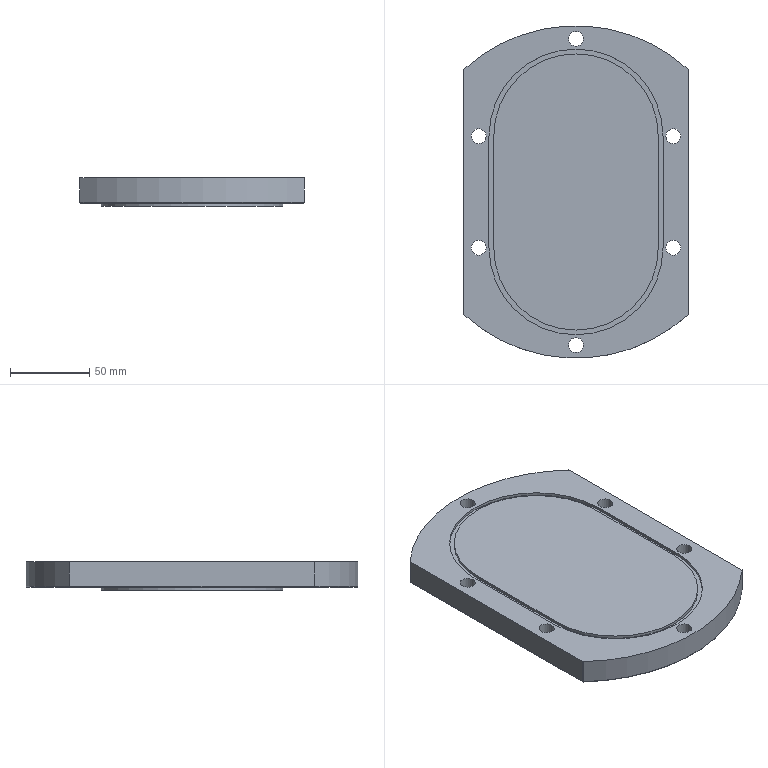NC program | NX | posted with a generic post | part box 142 x 210 x 18 mm
Whole program, first 1636 of 1921 lines:
N10 G17 G21 G94 G90
(FLOOR_WALL_COPY_1 , TOOL : D50)
N12 T02 M6
N14 G54
N16 G17 G0 G90 X-85.265 Y114.816 S1200 M3
N18 G43 Z30. H2
N20 Z7.65
N22 G94 G1 Z4.65 F1000.
N24 X-80.13
N26 X80.117 F2000.
N28 G2 X82.943 Y112.789 R139.395
N30 X115.013 Y79.847 R139.657
N32 G1 X-115.005
N34 G3 X-132.614 Y44.877 R139.395
N36 G1 X132.619
N38 G2 X135.762 Y34.188 R138.402
N40 X138.212 Y22.319 R138.876
N42 X139.185 Y15.081 R138.848
N44 G1 X139.188 Y15.055
N46 G2 X139.52 Y11.62 R138.455
N48 X139.654 Y9.908 R139.238
N50 G1 X-139.654
N52 G3 X-140. Y1.556 R138.451
N54 G1 Y-1.551
N56 G3 X-139.185 Y-15.081 R138.451
N58 X-139.096 Y-15.879 R138.876
N60 X-137.742 Y-25.061 R138.874
N62 G1 X137.753
N64 G2 X133.543 Y-42.026 R139.238
N66 G1 X133.535 Y-42.053
N68 G2 X126.487 Y-60.031 R139.394
N70 G1 X-126.475
N72 G3 X-102.857 Y-95. R139.108
N74 G1 X102.85
N76 X106.896
N78 Z7.65
N80 G0 Z30.
N82 X-85.278 Y114.807
N84 Z7.3
N86 G1 Z4.3 F1000.
N88 X-80.144
N90 X80.131 F2000.
N92 G2 X82.943 Y112.789 R139.395
N94 X88.4 Y108.57 R139.657
N96 X95.762 Y102.141 R139.226
N98 X115.019 Y79.839 R139.657
N100 G1 X-115.01
N102 G3 X-131.183 Y48.912 R139.395
N104 X-132.617 Y44.871 R139.232
N106 G1 X132.621
N108 G2 X133.663 Y41.664 R138.402
N110 X138.725 Y18.859 R139.471
N112 X139.177 Y15.15 R138.876
N114 X139.284 Y14.148 R138.613
N116 X139.654 Y9.903 R138.455
N118 G1 X-139.654
N120 G3 X-140. Y1.556 R138.452
N122 G1 Y-1.551
N124 G3 X-139.284 Y-14.144 R138.452
N126 X-139.177 Y-15.15 R138.609
N128 X-138.72 Y-18.899 R138.874
N130 X-137.742 Y-25.064 R139.469
N132 G1 X137.744
N134 G2 X133.556 Y-41.985 R138.547
N136 X131.173 Y-48.938 R139.231
N138 X126.486 Y-60.032 R139.394
N140 G1 X-126.494
N142 G3 X-102.838 Y-95. R140.983
N144 G1 X102.85
N146 X106.897
N148 Z7.3
N150 G0 Z30.
N152 X-85.269 Y114.807
N154 Z6.95
N156 G1 Z3.95 F1000.
N158 X-80.13
N160 X80.121 F2000.
N162 G2 X115.009 Y79.839 R139.149
N164 G1 X-115.002
N166 G3 X-115.739 Y78.769 R139.74
N168 X-128.743 Y55.02 R139.232
N170 X-132.622 Y44.871 R139.74
N172 G1 X132.62
N174 G2 X135.313 Y35.943 R139.471
N176 X139.159 Y15.32 R137.837
N178 X139.414 Y12.819 R138.939
N180 X139.653 Y9.903 R138.613
N182 G1 X-139.654
N184 G3 X-140. Y1.469 R138.609
N186 G1 Y-1.466
N188 G3 X-139.415 Y-12.808 R138.609
N190 X-139.159 Y-15.32 R138.939
N192 X-137.747 Y-25.064 R137.838
N194 G1 X137.742
N196 G2 X128.804 Y-54.879 R139.741
N198 X126.485 Y-60.032 R139.231
N200 G1 X-126.494
N202 G3 X-122.148 Y-68.39 R123.247
N204 X-118.721 Y-74.228 R123.999
N206 X-113.449 Y-82.027 R127.339
N208 X-103.593 Y-94.179 R130.009
N210 X-102.842 Y-95. R138.664
N212 G1 X102.854
N214 X106.901
N216 Z6.95
N218 G0 Z30.
N220 X-85.269 Y114.807
N222 Z6.6
N224 G1 Z3.6 F1000.
N226 X-80.13
N228 X80.122 F2000.
N230 G2 X83.799 Y112.156 R139.171
N232 X115.009 Y79.839 R139.149
N234 G1 X-115.003
N236 X-115.016 Y79.82
N238 G3 X-124.925 Y63.209 R138.142
N240 X-132.622 Y44.871 R139.74
N242 G1 X132.617
N244 G2 X133.643 Y41.704 R137.21
N246 X134.529 Y38.766 R138.012
N248 X138.955 Y17.095 R137.837
N250 X139.654 Y9.903 R139.66
N252 G1 X-139.656
N254 G3 X-140. Y1.365 R139.659
N256 G1 Y-1.337
N258 G3 X-138.954 Y-17.098 R139.659
N260 X-137.747 Y-25.064 R137.838
N262 G1 X137.742
N264 G2 X126.483 Y-60.032 R139.741
N266 G1 X-126.483
N268 G3 X-123.107 Y-66.674 R138.63
N270 G1 X-122.156 Y-68.375
N272 G3 X-117.49 Y-76.164 R122.385
N274 X-113.518 Y-81.933 R127.339
N276 X-102.859 Y-95. R136.562
N278 G1 X102.854
N280 X106.901
N282 Z6.6
N284 G0 Z30.
N286 X-85.266 Y114.806
N288 Z6.25
N290 G1 Z3.25 F1000.
N292 X-80.123
N294 X80.122 F2000.
N296 G2 X83.65 Y112.267 R139.171
N298 X115.004 Y79.839 R138.896
N300 G1 X-115.003
N302 X-115.016 Y79.82
N304 G3 X-123.362 Y66.212 R138.142
N306 X-130.723 Y50.13 R139.232
N308 X-132.622 Y44.871 R137.75
N310 G1 X132.621
N312 G2 X134.799 Y37.82 R138.521
N314 X138.659 Y19.342 R138.012
N316 X138.732 Y18.809 R138.88
N318 X139.654 Y9.903 R139.66
N320 G1 X-139.656
N322 G3 X-139.933 Y4.541 R139.659
N324 X-140. Y1.44 R138.722
N326 G1 Y-1.438
N328 G3 X-139.751 Y-8.435 R138.722
N330 X-138.732 Y-18.811 R139.659
N332 X-138.659 Y-19.343 R138.89
N334 X-137.744 Y-25.065 R138.022
N336 G1 X137.744
N338 G2 X134.714 Y-38.118 R138.502
N340 X130.724 Y-50.127 R137.741
N342 X126.485 Y-60.032 R139.231
N344 G1 X-126.483
N346 G3 X-102.859 Y-95. R139.597
N348 G1 X102.857
N350 X106.903
N352 Z6.25
N354 G0 Z30.
N356 X-85.265 Y114.807
N358 Z5.9
N360 G1 Z2.9 F1000.
N362 X-80.123
N364 X80.119 F2000.
N366 G2 X113.93 Y81.368 R138.88
N368 X115.004 Y79.839 R138.896
N370 G1 X-115.002
N372 G3 X-132.617 Y44.871 R139.233
N374 G1 X132.623
N376 G2 X139.118 Y15.686 R139.129
N378 X139.163 Y15.282 R138.88
N380 X139.446 Y12.465 R138.725
N382 X139.654 Y9.903 R138.455
N384 G1 X-139.654
N386 G3 X-140. Y1.558 R138.455
N388 G1 Y-1.552
N390 G3 X-139.45 Y-12.419 R138.455
N392 X-139.163 Y-15.282 R138.722
N394 X-139.115 Y-15.713 R138.89
N396 X-137.745 Y-25.064 R139.128
N398 G1 X137.744
N400 G2 X133.551 Y-42.002 R138.502
N402 X126.485 Y-60.032 R139.232
N404 G1 X-126.474
N406 G3 X-102.857 Y-95. R139.165
N408 G1 X102.857
N410 X106.903
N412 Z5.9
N414 G0 Z30.
N416 X-85.268 Y114.805
N418 Z5.55
N420 G1 Z2.55 F1000.
N422 X-80.125
N424 X80.122 F2000.
N426 G2 X80.507 Y114.536 R138.93
N428 X115.005 Y79.837 R138.88
N430 G1 X-115.003
N432 G3 X-132.617 Y44.87 R139.233
N434 G1 X132.623
N436 G2 X139.184 Y15.088 R139.129
N438 X139.278 Y14.2 R138.477
N440 X139.654 Y9.902 R138.455
N442 G1 X-139.654
N444 G3 X-140. Y1.558 R138.455
N446 G1 Y-1.552
N448 G3 X-139.28 Y-14.181 R138.455
N450 X-139.184 Y-15.088 R138.473
N452 X-137.745 Y-25.065 R139.128
N454 G1 X137.744
N456 G2 X133.854 Y-41.029 R138.519
N458 X133.55 Y-42.004 R138.632
N460 X126.485 Y-60.033 R139.232
N462 G1 X-126.474
N464 G3 X-102.838 Y-95. R139.809
N466 G1 X102.857
N468 X106.903
N470 Z5.55
N472 G0 Z30.
N474 X-85.264 Y114.807
N476 Z5.2
N478 G1 Z2.2 F1000.
N480 X-80.122
N482 X80.118 F2000.
N484 G2 X80.499 Y114.542 R139.232
N486 X115.003 Y79.839 R138.93
N488 G1 X-115.002
N490 G3 X-132.617 Y44.871 R139.23
N492 G1 X132.62
N494 G2 X133.452 Y42.333 R138.497
N496 X138.855 Y17.871 R139.483
N498 X139.176 Y15.162 R138.923
N500 X139.287 Y14.117 R138.616
N502 X139.654 Y9.904 R138.477
N504 G1 X-139.654
N506 G3 X-140. Y1.544 R138.474
N508 G1 Y-1.539
N510 G3 X-139.287 Y-14.113 R138.474
N512 X-139.176 Y-15.162 R138.612
N514 X-138.873 Y-17.736 R138.95
N516 X-137.742 Y-25.064 R139.482
N518 G1 X137.743
N520 G2 X133.554 Y-41.99 R138.632
N522 X126.485 Y-60.032 R139.229
N524 G1 X-126.494
N526 X-124.405 Y-64.245
N528 G3 X-102.838 Y-95. R141.78
N530 G1 X102.856
N532 X106.902
N534 Z5.2
N536 G0 Z30.
N538 X-85.284 Y114.807
N540 Z4.85
N542 G1 Z1.85 F1000.
N544 X-80.153
N546 X80.121 F2000.
N548 G2 X87.351 Y109.415 R137.487
N550 X103.242 Y94.574 R139.233
N552 X115.025 Y79.839 R139.49
N554 G1 X-115.002
N556 G3 X-115.982 Y78.411 R139.602
N558 X-129.013 Y54.385 R139.23
N560 X-132.621 Y44.871 R139.602
N562 G1 X132.62
N564 G2 X135.276 Y36.082 R139.483
N566 X139.159 Y15.323 R137.837
N568 X139.413 Y12.822 R138.93
N570 X139.653 Y9.903 R138.616
N572 G1 X-139.654
N574 G3 X-140. Y1.467 R138.612
N576 G1 Y-1.464
N578 G3 X-139.414 Y-12.81 R138.612
N580 X-139.159 Y-15.323 R138.93
N582 X-137.747 Y-25.064 R137.842
N584 G1 X137.741
N586 G2 X134.716 Y-38.112 R139.381
N588 X129.116 Y-54.14 R139.607
N590 X126.485 Y-60.032 R139.229
N592 G1 X-126.494
N594 G3 X-102.852 Y-95. R139.774
N596 G1 X102.85
N598 X106.897
N600 Z4.85
N602 G0 Z30.
N604 X-85.284 Y114.806
N606 Z4.5
N608 G1 Z1.5 F1000.
N610 X-80.153
N612 X80.127 F2000.
N614 G2 X84.771 Y111.424 R139.655
N616 X89.023 Y108.059 R137.487
N618 X99.219 Y98.78 R139.655
N620 X115.025 Y79.839 R139.49
N622 G1 X-115.007
N624 G3 X-117.111 Y76.717 R139.654
N626 X-124.145 Y64.728 R138.187
N628 X-131.551 Y47.919 R139.602
N630 X-132.622 Y44.871 R137.787
N632 G1 X132.622
N634 G2 X136.195 Y32.456 R139.162
N636 X138.955 Y17.095 R137.837
N638 X139.654 Y9.903 R139.66
N640 G1 X-139.656
N642 G3 X-140. Y1.364 R139.659
N644 G1 Y-1.336
N646 G3 X-138.954 Y-17.1 R139.659
N648 X-137.747 Y-25.065 R137.842
N650 G1 X137.742
N652 G2 X137.7 Y-25.289 R139.66
N654 X134.716 Y-38.112 R139.381
N656 X134.606 Y-38.501 R139.607
N658 X131.512 Y-48.025 R137.779
N660 X126.483 Y-60.032 R139.607
N662 G1 X-126.495
N664 G3 X-102.859 Y-95. R139.917
N666 G1 X102.844
N668 X106.892
N670 Z4.5
N672 G0 Z30.
N674 X-85.266 Y114.806
N676 Z4.15
N678 G1 Z1.15 F1000.
N680 X-80.123
N682 X80.127 F2000.
N684 G2 X83.869 Y112.104 R139.655
N686 X115.004 Y79.839 R138.88
N688 G1 X-115.007
N690 G3 X-117.031 Y76.838 R139.654
N692 X-117.476 Y76.157 R139.232
N694 X-121.948 Y68.779 R138.187
N696 X-130.666 Y50.278 R139.232
N698 X-132.622 Y44.871 R137.787
N700 G1 X132.622
N702 G2 X138.664 Y19.307 R139.162
N704 X138.715 Y18.936 R138.844
N706 X139.654 Y9.903 R139.66
N708 G1 X-139.656
N710 G3 X-139.921 Y4.893 R139.659
N712 X-140. Y1.449 R138.653
N714 G1 Y-1.443
N716 G3 X-139.779 Y-7.956 R138.653
N718 X-138.714 Y-18.944 R139.659
N720 X-138.666 Y-19.291 R138.851
N722 X-137.744 Y-25.065 R139.161
N724 G1 X137.744
N726 G2 X134.714 Y-38.118 R138.448
N728 X130.667 Y-50.275 R137.779
N730 X126.485 Y-60.032 R139.231
N732 G1 X-126.495
N734 G3 X-102.859 Y-95. R139.994
N736 G1 X102.857
N738 X106.903
N740 Z4.15
N742 G0 Z30.
N744 X-85.265 Y114.807
N746 Z3.8
N748 G1 Z0.8 F1000.
N750 X-80.123
N752 X80.119 F2000.
N754 G2 X82.841 Y112.864 R138.88
N756 X115.004 Y79.839 R138.88
N758 G1 X-115.002
N760 G3 X-132.617 Y44.871 R139.232
N762 G1 X132.621
N764 G2 X135.036 Y36.961 R138.401
N766 X135.767 Y34.171 R138.522
N768 X139.184 Y15.088 R138.844
N770 G1 X139.185 Y15.081
N772 G2 X139.654 Y9.903 R138.455
N774 G1 X-139.654
N776 G3 X-140. Y1.558 R138.455
N778 G1 Y-1.552
N780 G3 X-139.185 Y-15.081 R138.455
N782 G1 X-139.184 Y-15.087
N784 G3 X-137.741 Y-25.064 R138.852
N786 G1 X137.744
N788 G2 X133.535 Y-42.053 R138.448
N790 X126.485 Y-60.032 R139.231
N792 G1 X-126.474
N794 G3 X-102.852 Y-95. R139.21
N796 G1 X102.857
N798 X106.903
N800 Z3.8
N802 G0 Z30.
N804 X-85.269 Y114.804
N806 Z3.45
N808 G1 Z0.45 F1000.
N810 X-80.127
N812 X80.123 F2000.
N814 G2 X80.545 Y114.509 R138.938
N816 X115.005 Y79.837 R138.88
N818 G1 X-115.003
N820 G3 X-132.617 Y44.869 R139.232
N822 G1 X132.621
N824 G2 X135.763 Y34.187 R138.401
N826 X139.183 Y15.092 R138.873
N828 X139.278 Y14.207 R138.483
N830 X139.654 Y9.902 R138.455
N832 G1 X-139.654
N834 G3 X-140. Y1.558 R138.455
N836 G1 Y-1.552
N838 G3 X-139.279 Y-14.196 R138.455
N840 X-139.183 Y-15.092 R138.48
N842 X-137.741 Y-25.065 R138.874
N844 G1 X137.743
N846 G2 X133.535 Y-42.053 R138.545
N848 X126.485 Y-60.033 R139.231
N850 G1 X-126.494
N852 G3 X-113.384 Y-82.122 R138.552
N854 G1 X-112.383 Y-83.497
N856 X-109.545 Y-87.203
N858 X-106.577 Y-90.805
N860 X-102.838 Y-95.
N862 X102.857
N864 X106.903
N866 Z3.45
N868 G0 Z30.
N870 X-85.264 Y114.807
N872 Z3.1
N874 G1 Z0.1 F1000.
N876 X-80.121
N878 X80.118 F2000.
N880 G2 X80.494 Y114.545 R139.255
N882 X115.003 Y79.839 R138.938
N884 G1 X-115.001
N886 G3 X-132.617 Y44.872 R139.226
N888 G1 X132.62
N890 G2 X134.736 Y38.044 R138.475
N892 X139.166 Y15.256 R137.63
N894 G1 X139.175 Y15.166
N896 G2 X139.286 Y14.126 R138.625
N898 X139.654 Y9.904 R138.483
N900 G1 X-139.654
N902 G3 X-140. Y1.54 R138.48
N904 G1 Y-1.535
N906 G3 X-139.292 Y-14.064 R138.48
N908 X-139.167 Y-15.247 R138.624
N910 X-137.748 Y-25.064 R137.636
N912 G1 X137.743
N914 G2 X133.565 Y-41.958 R138.622
N916 X126.485 Y-60.032 R139.225
N918 G1 X-126.494
N920 G3 X-102.838 Y-95. R140.977
N922 G1 X102.856
N924 X106.902
N926 Z3.1
N928 G0 Z30.
(FLOOR_WALL_COPY_COPY , TOOL : D50)
N930 X-85.265 Y114.816 S2500
N932 Z3.
N934 G1 Z0. F1000.
N936 X-80.13
N938 X80.117
N940 G2 X82.943 Y112.789 R139.395
N942 X115.013 Y79.847 R139.657
N944 G1 X-115.005
N946 G3 X-132.614 Y44.877 R139.395
N948 G1 X132.619
N950 G2 X135.762 Y34.188 R138.402
N952 X138.259 Y22.023 R138.881
N954 X138.818 Y18.164 R138.848
N956 X139.184 Y15.083 R138.881
N958 X139.484 Y12.039 R139.242
N960 X139.654 Y9.908 R139.238
N962 G1 X-139.654
N964 G3 X-140. Y1.556 R138.451
N966 G1 Y-1.551
N968 G3 X-139.483 Y-12.048 R138.451
N970 X-139.184 Y-15.082 R138.46
N972 X-137.742 Y-25.061 R138.879
N974 G1 X137.753
N976 G2 X133.75 Y-41.364 R139.238
N978 X133.535 Y-42.053 R139.242
N980 X126.487 Y-60.031 R139.394
N982 G1 X-126.475
N984 G3 X-102.857 Y-95. R139.178
N986 G1 X102.85
N988 X106.896
N990 Z3.
N992 G0 Z30.
N994 M5
(DRILLING , TOOL : ZXZ)
N996 T01 M6
N998 G54
N1000 G17 G0 G90 X96.75 Y0. S5000 M3
N1002 G43 Z30. H1
N1004 G94 G81 G98 Z-1. F250. R3.
N1006 X35.25 Y-61.5
N1008 Y61.5
N1010 X-35.25
N1012 Y-61.5
N1014 X-96.75 Y0.
N1016 G80
N1018 G0 X-96.75 Y0. Z30.
N1020 M5
(DRILLING_COPY , TOOL : 9.5ZT)
N1022 T09 M6
N1024 G54
N1026 G17 G0 G90 X96.75 Y0. S2000 M3
N1028 G43 Z30. H9
N1030 G94 G83 G98 Z-21.854 F200. Q2. R3.
N1032 X35.25 Y-61.5
N1034 Y61.5
N1036 X-35.25
N1038 Y-61.5
N1040 X-96.75 Y0.
N1042 G80
N1044 G0 X-96.75 Y0. Z30.
N1046 M5
(PLANAR_PROFILE , TOOL : D3)
N1048 T03 M6
N1050 G54
N1052 G17 G0 G90 X0. Y53.5 S5000 M3
N1054 G43 Z30. H3
N1056 Z3.
N1058 G94 G1 Z-0.05 F500.
N1060 X-35.25 F1100.
N1062 G3 X-88.75 Y0. R53.5
N1064 X-35.25 Y-53.5 R53.5
N1066 G1 X35.25
N1068 G3 X88.75 Y0. R53.5
N1070 X35.25 Y53.5 R53.5
N1072 G1 X0.
N1074 Z2.95
N1076 Z-0.1 F500.
N1078 X35.25 F1100.
N1080 G2 X88.75 Y0. R53.5
N1082 X35.25 Y-53.5 R53.5
N1084 G1 X-35.25
N1086 G2 X-88.75 Y0. R53.5
N1088 X-35.25 Y53.5 R53.5
N1090 G1 X0.
N1092 Z2.9
N1094 Z-0.15 F500.
N1096 X-35.25 F1100.
N1098 G3 X-88.75 Y0. R53.5
N1100 X-35.25 Y-53.5 R53.5
N1102 G1 X35.25
N1104 G3 X88.75 Y0. R53.5
N1106 X35.25 Y53.5 R53.5
N1108 G1 X0.
N1110 Z2.85
N1112 Z-0.2 F500.
N1114 X35.25 F1100.
N1116 G2 X88.75 Y0. R53.5
N1118 X35.25 Y-53.5 R53.5
N1120 G1 X-35.25
N1122 G2 X-88.75 Y0. R53.5
N1124 X-35.25 Y53.5 R53.5
N1126 G1 X0.
N1128 Z2.8
N1130 Z-0.25 F500.
N1132 X-35.25 F1100.
N1134 G3 X-88.75 Y0. R53.5
N1136 X-35.25 Y-53.5 R53.5
N1138 G1 X35.25
N1140 G3 X88.75 Y0. R53.5
N1142 X35.25 Y53.5 R53.5
N1144 G1 X0.
N1146 Z2.75
N1148 Z-0.3 F500.
N1150 X35.25 F1100.
N1152 G2 X88.75 Y0. R53.5
N1154 X35.25 Y-53.5 R53.5
N1156 G1 X-35.25
N1158 G2 X-88.75 Y0. R53.5
N1160 X-35.25 Y53.5 R53.5
N1162 G1 X0.
N1164 Z2.7
N1166 Z-0.35 F500.
N1168 X-35.25 F1100.
N1170 G3 X-88.75 Y0. R53.5
N1172 X-35.25 Y-53.5 R53.5
N1174 G1 X35.25
N1176 G3 X88.75 Y0. R53.5
N1178 X35.25 Y53.5 R53.5
N1180 G1 X0.
N1182 Z2.65
N1184 Z-0.4 F500.
N1186 X35.25 F1100.
N1188 G2 X88.75 Y0. R53.5
N1190 X35.25 Y-53.5 R53.5
N1192 G1 X-35.25
N1194 G2 X-88.75 Y0. R53.5
N1196 X-35.25 Y53.5 R53.5
N1198 G1 X0.
N1200 Z2.6
N1202 Z-0.45 F500.
N1204 X-35.25 F1100.
N1206 G3 X-88.75 Y0. R53.5
N1208 X-35.25 Y-53.5 R53.5
N1210 G1 X35.25
N1212 G3 X88.75 Y0. R53.5
N1214 X35.25 Y53.5 R53.5
N1216 G1 X0.
N1218 Z2.55
N1220 Z-0.5 F500.
N1222 X35.25 F1100.
N1224 G2 X88.75 Y0. R53.5
N1226 X35.25 Y-53.5 R53.5
N1228 G1 X-35.25
N1230 G2 X-88.75 Y0. R53.5
N1232 X-35.25 Y53.5 R53.5
N1234 G1 X0.
N1236 Z2.5
N1238 Z-0.55 F500.
N1240 X-35.25 F1100.
N1242 G3 X-88.75 Y0. R53.5
N1244 X-35.25 Y-53.5 R53.5
N1246 G1 X35.25
N1248 G3 X88.75 Y0. R53.5
N1250 X35.25 Y53.5 R53.5
N1252 G1 X0.
N1254 Z2.45
N1256 Z-0.6 F500.
N1258 X35.25 F1100.
N1260 G2 X88.75 Y0. R53.5
N1262 X35.25 Y-53.5 R53.5
N1264 G1 X-35.25
N1266 G2 X-88.75 Y0. R53.5
N1268 X-35.25 Y53.5 R53.5
N1270 G1 X0.
N1272 Z2.4
N1274 Z-0.65 F500.
N1276 X-35.25 F1100.
N1278 G3 X-88.75 Y0. R53.5
N1280 X-35.25 Y-53.5 R53.5
N1282 G1 X35.25
N1284 G3 X88.75 Y0. R53.5
N1286 X35.25 Y53.5 R53.5
N1288 G1 X0.
N1290 Z2.35
N1292 Z-0.7 F500.
N1294 X35.25 F1100.
N1296 G2 X88.75 Y0. R53.5
N1298 X35.25 Y-53.5 R53.5
N1300 G1 X-35.25
N1302 G2 X-88.75 Y0. R53.5
N1304 X-35.25 Y53.5 R53.5
N1306 G1 X0.
N1308 Z2.3
N1310 Z-0.75 F500.
N1312 X-35.25 F1100.
N1314 G3 X-88.75 Y0. R53.5
N1316 X-35.25 Y-53.5 R53.5
N1318 G1 X35.25
N1320 G3 X88.75 Y0. R53.5
N1322 X35.25 Y53.5 R53.5
N1324 G1 X0.
N1326 Z2.25
N1328 Z-0.8 F500.
N1330 X35.25 F1100.
N1332 G2 X88.75 Y0. R53.5
N1334 X35.25 Y-53.5 R53.5
N1336 G1 X-35.25
N1338 G2 X-88.75 Y0. R53.5
N1340 X-35.25 Y53.5 R53.5
N1342 G1 X0.
N1344 Z2.2
N1346 Z-0.85 F500.
N1348 X-35.25 F1100.
N1350 G3 X-88.75 Y0. R53.5
N1352 X-35.25 Y-53.5 R53.5
N1354 G1 X35.25
N1356 G3 X88.75 Y0. R53.5
N1358 X35.25 Y53.5 R53.5
N1360 G1 X0.
N1362 Z2.15
N1364 Z-0.9 F500.
N1366 X35.25 F1100.
N1368 G2 X88.75 Y0. R53.5
N1370 X35.25 Y-53.5 R53.5
N1372 G1 X-35.25
N1374 G2 X-88.75 Y0. R53.5
N1376 X-35.25 Y53.5 R53.5
N1378 G1 X0.
N1380 Z2.1
N1382 Z-0.95 F500.
N1384 X-35.25 F1100.
N1386 G3 X-88.75 Y0. R53.5
N1388 X-35.25 Y-53.5 R53.5
N1390 G1 X35.25
N1392 G3 X88.75 Y0. R53.5
N1394 X35.25 Y53.5 R53.5
N1396 G1 X0.
N1398 Z2.05
N1400 Z-1. F500.
N1402 X35.25 F1100.
N1404 G2 X88.75 Y0. R53.5
N1406 X35.25 Y-53.5 R53.5
N1408 G1 X-35.25
N1410 G2 X-88.75 Y0. R53.5
N1412 X-35.25 Y53.5 R53.5
N1414 G1 X0.
N1416 Z2.
N1418 Z-1.05 F500.
N1420 X-35.25 F1100.
N1422 G3 X-88.75 Y0. R53.5
N1424 X-35.25 Y-53.5 R53.5
N1426 G1 X35.25
N1428 G3 X88.75 Y0. R53.5
N1430 X35.25 Y53.5 R53.5
N1432 G1 X0.
N1434 Z1.95
N1436 Z-1.1 F500.
N1438 X35.25 F1100.
N1440 G2 X88.75 Y0. R53.5
N1442 X35.25 Y-53.5 R53.5
N1444 G1 X-35.25
N1446 G2 X-88.75 Y0. R53.5
N1448 X-35.25 Y53.5 R53.5
N1450 G1 X0.
N1452 Z1.9
N1454 Z-1.15 F500.
N1456 X-35.25 F1100.
N1458 G3 X-88.75 Y0. R53.5
N1460 X-35.25 Y-53.5 R53.5
N1462 G1 X35.25
N1464 G3 X88.75 Y0. R53.5
N1466 X35.25 Y53.5 R53.5
N1468 G1 X0.
N1470 Z1.85
N1472 Z-1.2 F500.
N1474 X35.25 F1100.
N1476 G2 X88.75 Y0. R53.5
N1478 X35.25 Y-53.5 R53.5
N1480 G1 X-35.25
N1482 G2 X-88.75 Y0. R53.5
N1484 X-35.25 Y53.5 R53.5
N1486 G1 X0.
N1488 Z1.8
N1490 Z-1.25 F500.
N1492 X-35.25 F1100.
N1494 G3 X-88.75 Y0. R53.5
N1496 X-35.25 Y-53.5 R53.5
N1498 G1 X35.25
N1500 G3 X88.75 Y0. R53.5
N1502 X35.25 Y53.5 R53.5
N1504 G1 X0.
N1506 Z1.75
N1508 Z-1.3 F500.
N1510 X35.25 F1100.
N1512 G2 X88.75 Y0. R53.5
N1514 X35.25 Y-53.5 R53.5
N1516 G1 X-35.25
N1518 G2 X-88.75 Y0. R53.5
N1520 X-35.25 Y53.5 R53.5
N1522 G1 X0.
N1524 Z1.7
N1526 Z-1.35 F500.
N1528 X-35.25 F1100.
N1530 G3 X-88.75 Y0. R53.5
N1532 X-35.25 Y-53.5 R53.5
N1534 G1 X35.25
N1536 G3 X88.75 Y0. R53.5
N1538 X35.25 Y53.5 R53.5
N1540 G1 X0.
N1542 Z1.65
N1544 Z-1.4 F500.
N1546 X35.25 F1100.
N1548 G2 X88.75 Y0. R53.5
N1550 X35.25 Y-53.5 R53.5
N1552 G1 X-35.25
N1554 G2 X-88.75 Y0. R53.5
N1556 X-35.25 Y53.5 R53.5
N1558 G1 X0.
N1560 Z1.6
N1562 Z-1.45 F500.
N1564 X-35.25 F1100.
N1566 G3 X-88.75 Y0. R53.5
N1568 X-35.25 Y-53.5 R53.5
N1570 G1 X35.25
N1572 G3 X88.75 Y0. R53.5
N1574 X35.25 Y53.5 R53.5
N1576 G1 X0.
N1578 Z1.55
N1580 Z-1.5 F500.
N1582 X35.25 F1100.
N1584 G2 X88.75 Y0. R53.5
N1586 X35.25 Y-53.5 R53.5
N1588 G1 X-35.25
N1590 G2 X-88.75 Y0. R53.5
N1592 X-35.25 Y53.5 R53.5
N1594 G1 X0.
N1596 Z1.5
N1598 Z-1.55 F500.
N1600 X-35.25 F1100.
N1602 G3 X-88.75 Y0. R53.5
N1604 X-35.25 Y-53.5 R53.5
N1606 G1 X35.25
N1608 G3 X88.75 Y0. R53.5
N1610 X35.25 Y53.5 R53.5
N1612 G1 X0.
N1614 Z1.45
N1616 Z-1.6 F500.
N1618 X35.25 F1100.
N1620 G2 X88.75 Y0. R53.5
N1622 X35.25 Y-53.5 R53.5
N1624 G1 X-35.25
N1626 G2 X-88.75 Y0. R53.5
N1628 X-35.25 Y53.5 R53.5
N1630 G1 X0.
N1632 Z1.4
N1634 Z-1.65 F500.
N1636 X-35.25 F1100.
N1638 G3 X-88.75 Y0. R53.5
N1640 X-35.25 Y-53.5 R53.5
N1642 G1 X35.25
N1644 G3 X88.75 Y0. R53.5
N1646 X35.25 Y53.5 R53.5
N1648 G1 X0.
N1650 Z1.35
N1652 Z-1.7 F500.
N1654 X35.25 F1100.
N1656 G2 X88.75 Y0. R53.5
N1658 X35.25 Y-53.5 R53.5
N1660 G1 X-35.25
N1662 G2 X-88.75 Y0. R53.5
N1664 X-35.25 Y53.5 R53.5
N1666 G1 X0.
N1668 Z1.3
N1670 Z-1.75 F500.
N1672 X-35.25 F1100.
N1674 G3 X-88.75 Y0. R53.5
N1676 X-35.25 Y-53.5 R53.5
N1678 G1 X35.25
N1680 G3 X88.75 Y0. R53.5
N1682 X35.25 Y53.5 R53.5
N1684 G1 X0.
N1686 Z1.25
N1688 Z-1.8 F500.
N1690 X35.25 F1100.
N1692 G2 X88.75 Y0. R53.5
N1694 X35.25 Y-53.5 R53.5
N1696 G1 X-35.25
N1698 G2 X-88.75 Y0. R53.5
N1700 X-35.25 Y53.5 R53.5
N1702 G1 X0.
N1704 Z1.2
N1706 G0 Z30.
N1708 M5
(ZLEVEL_PROFILE_COPY , TOOL : D25R0.5)
N1710 T05 M6
N1712 G54
N1714 G17 G0 G90 X-85.417 Y92.764 S2000 M3
N1716 G43 Z30. H5
N1718 Z-0.35
N1720 G94 G1 X-80.908 Y84.905 F1000.
N1722 G3 X-78.747 Y83.649 R2.5
N1724 G1 X-78.136 Y83.647 F2200.
N1726 X-76.916
N1728 X-73.1 Y83.65
N1730 X77.154 Y83.649
N1732 X78.136 Y83.647
N1734 X78.747 Y83.649
N1736 G3 X80.908 Y84.905 R2.5
N1738 G1 X85.417 Y92.764
N1740 X-85.403 Y92.767 Z-0.7
N1742 X-80.907 Y84.908 F1000.
N1744 G3 X-78.747 Y83.649 R2.5
N1746 G1 X-77.526 Y83.644 F2200.
N1748 X-73.1 Y83.65
N1750 X77.172
N1752 G2 X77.526 Y83.644 R13.15
N1754 G1 X78.747 Y83.649
N1756 G3 X80.907 Y84.908 R2.5
N1758 G1 X85.403 Y92.767
N1760 X-85.403 Y92.768 Z-1.05
N1762 X-80.907 Y84.908 F1000.
N1764 G3 X-78.747 Y83.649 R2.5
N1766 G1 X-77.526 Y83.644 F2200.
N1768 X-73.1 Y83.65
N1770 X77.172
N1772 G2 X77.526 Y83.644 R13.15
N1774 G1 X78.747 Y83.649
N1776 G3 X80.907 Y84.908 R2.5
N1778 G1 X85.403 Y92.768
N1780 X-85.403 Z-1.4
N1782 X-80.907 Y84.908 F1000.
N1784 G3 X-78.747 Y83.649 R2.5
N1786 G1 X-77.526 Y83.644 F2200.
N1788 X-73.1 Y83.65
N1790 X77.172
N1792 G2 X77.526 Y83.644 R13.15
N1794 G1 X78.747 Y83.649
N1796 G3 X80.907 Y84.908 R2.5
N1798 G1 X85.403 Y92.768
N1800 X-85.403 Z-1.75
N1802 X-80.907 Y84.908 F1000.
N1804 G3 X-78.747 Y83.649 R2.5
N1806 G1 X-77.526 Y83.644 F2200.
N1808 X-73.1 Y83.65
N1810 X77.172
N1812 G2 X77.526 Y83.644 R13.15
N1814 G1 X78.747 Y83.649
N1816 G3 X80.907 Y84.908 R2.5
N1818 G1 X85.403 Y92.768
N1820 X-85.403 Z-2.1
N1822 X-80.907 Y84.908 F1000.
N1824 G3 X-78.747 Y83.649 R2.5
N1826 G1 X-77.526 Y83.644 F2200.
N1828 X-73.1 Y83.65
N1830 X77.172
N1832 G2 X77.526 Y83.644 R13.15
N1834 G1 X78.747 Y83.649
N1836 G3 X80.907 Y84.908 R2.5
N1838 G1 X85.403 Y92.768
N1840 X-85.403 Z-2.45
N1842 X-80.907 Y84.908 F1000.
N1844 G3 X-78.747 Y83.649 R2.5
N1846 G1 X-77.526 Y83.644 F2200.
N1848 X-73.1 Y83.65
N1850 X77.172
N1852 G2 X77.526 Y83.644 R13.15
N1854 G1 X78.747 Y83.649
N1856 G3 X80.907 Y84.908 R2.5
N1858 G1 X85.403 Y92.768
N1860 X-85.403 Z-2.8
N1862 X-80.907 Y84.908 F1000.
N1864 G3 X-78.747 Y83.649 R2.5
N1866 G1 X-77.526 Y83.644 F2200.
N1868 X-73.1 Y83.65
N1870 X77.172
N1872 G2 X77.526 Y83.644 R13.15
N1874 G1 X78.747 Y83.649
N1876 G3 X80.907 Y84.908 R2.5
N1878 G1 X85.403 Y92.768
N1880 X-85.402 Z-3.15
N1882 X-80.907 Y84.908 F1000.
N1884 G3 X-78.747 Y83.649 R2.5
N1886 G1 X-77.526 Y83.644 F2200.
N1888 X-73.1 Y83.65
N1890 X77.172
N1892 G2 X77.526 Y83.644 R13.15
N1894 G1 X78.747 Y83.649
N1896 G3 X80.907 Y84.908 R2.5
N1898 G1 X85.402 Y92.768
N1900 X-85.402 Z-3.5
N1902 X-80.907 Y84.908 F1000.
N1904 G3 X-78.747 Y83.649 R2.5
N1906 G1 X-77.526 Y83.644 F2200.
N1908 X-73.1 Y83.65
N1910 X77.172
N1912 G2 X77.526 Y83.644 R13.15
N1914 G1 X78.747 Y83.649
N1916 G3 X80.907 Y84.908 R2.5
N1918 G1 X85.402 Y92.768
N1920 X-85.402 Z-3.85
N1922 X-80.907 Y84.908 F1000.
N1924 G3 X-78.747 Y83.649 R2.5
N1926 G1 X-77.526 Y83.644 F2200.
N1928 X-73.1 Y83.65
N1930 X77.172
N1932 G2 X77.526 Y83.644 R13.15
N1934 G1 X78.747 Y83.649
N1936 G3 X80.907 Y84.908 R2.5
N1938 G1 X85.402 Y92.768
N1940 X-85.402 Z-4.2
N1942 X-80.907 Y84.908 F1000.
N1944 G3 X-78.747 Y83.649 R2.5
N1946 G1 X-77.526 Y83.644 F2200.
N1948 X-73.1 Y83.65
N1950 X77.172
N1952 G2 X77.526 Y83.644 R13.15
N1954 G1 X78.747 Y83.649
N1956 G3 X80.907 Y84.908 R2.5
N1958 G1 X85.402 Y92.768
N1960 X-85.402 Z-4.55
N1962 X-80.907 Y84.908 F1000.
N1964 G3 X-78.747 Y83.649 R2.5
N1966 G1 X-77.526 Y83.644 F2200.
N1968 X-73.1 Y83.65
N1970 X77.172
N1972 G2 X77.526 Y83.644 R13.15
N1974 G1 X78.747 Y83.649
N1976 G3 X80.907 Y84.908 R2.5
N1978 G1 X85.402 Y92.768
N1980 X-85.402 Z-4.9
N1982 X-80.907 Y84.908 F1000.
N1984 G3 X-78.747 Y83.649 R2.5
N1986 G1 X-77.526 Y83.644 F2200.
N1988 X-73.1 Y83.65
N1990 X77.172
N1992 G2 X77.526 Y83.644 R13.15
N1994 G1 X78.747 Y83.649
N1996 G3 X80.907 Y84.908 R2.5
N1998 G1 X85.402 Y92.768
N2000 X-85.402 Z-5.25
N2002 X-80.907 Y84.908 F1000.
N2004 G3 X-78.747 Y83.649 R2.5
N2006 G1 X-77.526 Y83.644 F2200.
N2008 X-73.1 Y83.65
N2010 X77.172
N2012 G2 X77.526 Y83.644 R13.15
N2014 G1 X78.747 Y83.649
N2016 G3 X80.907 Y84.908 R2.5
N2018 G1 X85.402 Y92.768
N2020 X-85.402 Z-5.6
N2022 X-80.907 Y84.908 F1000.
N2024 G3 X-78.747 Y83.649 R2.5
N2026 G1 X-77.526 Y83.644 F2200.
N2028 X-73.1 Y83.65
N2030 X77.172
N2032 G2 X77.526 Y83.644 R13.15
N2034 G1 X78.747 Y83.649
N2036 G3 X80.907 Y84.908 R2.5
N2038 G1 X85.402 Y92.768
N2040 X-85.402 Z-5.95
N2042 X-80.907 Y84.908 F1000.
N2044 G3 X-78.747 Y83.649 R2.5
N2046 G1 X-77.526 Y83.644 F2200.
N2048 X-73.1 Y83.65
N2050 X77.172
N2052 G2 X77.526 Y83.644 R13.15
N2054 G1 X78.747 Y83.649
N2056 G3 X80.907 Y84.908 R2.5
N2058 G1 X85.402 Y92.768
N2060 X-85.401 Z-6.3
N2062 X-80.907 Y84.908 F1000.
N2064 G3 X-78.747 Y83.649 R2.5
N2066 G1 X-77.526 Y83.644 F2200.
N2068 X-73.1 Y83.65
N2070 X77.172
N2072 G2 X77.526 Y83.644 R13.15
N2074 G1 X78.747 Y83.649
N2076 G3 X80.907 Y84.908 R2.5
N2078 G1 X85.401 Y92.768
N2080 X-85.401 Z-6.65
N2082 X-80.907 Y84.908 F1000.
N2084 G3 X-78.747 Y83.649 R2.5
N2086 G1 X-77.526 Y83.644 F2200.
N2088 X-73.1 Y83.65
N2090 X77.172
N2092 G2 X77.526 Y83.644 R13.15
N2094 G1 X78.747 Y83.649
N2096 G3 X80.907 Y84.908 R2.5
N2098 G1 X85.401 Y92.768
N2100 X-85.401 Z-7.
N2102 X-80.907 Y84.908 F1000.
N2104 G3 X-78.747 Y83.649 R2.5
N2106 G1 X-77.526 Y83.644 F2200.
N2108 X-73.1 Y83.65
N2110 X77.172
N2112 G2 X77.526 Y83.644 R13.15
N2114 G1 X78.747 Y83.649
N2116 G3 X80.907 Y84.908 R2.5
N2118 G1 X85.401 Y92.768
N2120 X-85.401 Z-7.35
N2122 X-80.907 Y84.908 F1000.
N2124 G3 X-78.747 Y83.649 R2.5
N2126 G1 X-77.526 Y83.644 F2200.
N2128 X-73.1 Y83.65
N2130 X77.172
N2132 G2 X77.526 Y83.644 R13.15
N2134 G1 X78.747 Y83.649
N2136 G3 X80.907 Y84.908 R2.5
N2138 G1 X85.401 Y92.768
N2140 X-85.401 Z-7.7
N2142 X-80.907 Y84.908 F1000.
N2144 G3 X-78.747 Y83.649 R2.5
N2146 G1 X-77.526 Y83.644 F2200.
N2148 X-73.1 Y83.65
N2150 X77.172
N2152 G2 X77.526 Y83.644 R13.15
N2154 G1 X78.747 Y83.649
N2156 G3 X80.907 Y84.908 R2.5
N2158 G1 X85.401 Y92.768
N2160 X-85.401 Z-8.05
N2162 X-80.907 Y84.908 F1000.
N2164 G3 X-78.747 Y83.649 R2.5
N2166 G1 X-77.526 Y83.644 F2200.
N2168 X-73.1 Y83.65
N2170 X77.172
N2172 G2 X77.526 Y83.644 R13.15
N2174 G1 X78.747 Y83.649
N2176 G3 X80.907 Y84.908 R2.5
N2178 G1 X85.401 Y92.768
N2180 X-85.401 Y92.769 Z-8.4
N2182 X-80.907 Y84.908 F1000.
N2184 G3 X-78.747 Y83.649 R2.5
N2186 G1 X-77.526 Y83.644 F2200.
N2188 X-73.1 Y83.65
N2190 X77.172
N2192 G2 X77.526 Y83.644 R13.15
N2194 G1 X78.747 Y83.649
N2196 G3 X80.907 Y84.908 R2.5
N2198 G1 X85.401 Y92.769
N2200 X-85.401 Z-8.75
N2202 X-80.907 Y84.909 F1000.
N2204 G3 X-78.747 Y83.649 R2.5
N2206 G1 X-77.526 Y83.644 F2200.
N2208 X-73.1 Y83.65
N2210 X77.172
N2212 G2 X77.526 Y83.644 R13.15
N2214 G1 X78.747 Y83.649
N2216 G3 X80.907 Y84.909 R2.5
N2218 G1 X85.401 Y92.769
N2220 X-85.4 Z-9.1
N2222 X-80.907 Y84.909 F1000.
N2224 G3 X-78.747 Y83.649 R2.5
N2226 G1 X-77.526 Y83.644 F2200.
N2228 X-73.1 Y83.65
N2230 X77.172
N2232 G2 X77.526 Y83.644 R13.15
N2234 G1 X78.747 Y83.649
N2236 G3 X80.907 Y84.909 R2.5
N2238 G1 X85.4 Y92.769
N2240 X-85.4 Z-9.45
N2242 X-80.907 Y84.909 F1000.
N2244 G3 X-78.747 Y83.649 R2.5
N2246 G1 X-77.526 Y83.644 F2200.
N2248 X-73.1 Y83.65
N2250 X77.172
N2252 G2 X77.526 Y83.644 R13.15
N2254 G1 X78.747 Y83.649
N2256 G3 X80.907 Y84.909 R2.5
N2258 G1 X85.4 Y92.769
N2260 X-85.4 Z-9.8
N2262 X-80.907 Y84.909 F1000.
N2264 G3 X-78.747 Y83.649 R2.5
N2266 G1 X-77.526 Y83.644 F2200.
N2268 X-73.1 Y83.65
N2270 X77.172
N2272 G2 X77.526 Y83.644 R13.15
N2274 G1 X78.747 Y83.649
N2276 G3 X80.907 Y84.909 R2.5
N2278 G1 X85.4 Y92.769
N2280 X-85.4 Z-10.15
N2282 X-80.907 Y84.909 F1000.
N2284 G3 X-78.747 Y83.649 R2.5
N2286 G1 X-77.526 Y83.644 F2200.
N2288 X-73.1 Y83.65
N2290 X77.172
N2292 G2 X77.526 Y83.644 R13.15
N2294 G1 X78.747 Y83.649
N2296 G3 X80.907 Y84.909 R2.5
N2298 G1 X85.4 Y92.769
N2300 X-85.4 Z-10.5
N2302 X-80.907 Y84.909 F1000.
N2304 G3 X-78.747 Y83.649 R2.5
N2306 G1 X-77.526 Y83.644 F2200.
N2308 X-73.1 Y83.65
N2310 X77.172
N2312 G2 X77.526 Y83.644 R13.15
N2314 G1 X78.747 Y83.649
N2316 G3 X80.907 Y84.909 R2.5
N2318 G1 X85.4 Y92.769
N2320 X-85.4 Z-10.85
N2322 X-80.907 Y84.909 F1000.
N2324 G3 X-78.747 Y83.649 R2.5
N2326 G1 X-77.526 Y83.644 F2200.
N2328 X-73.1 Y83.65
N2330 X77.172
N2332 G2 X77.526 Y83.644 R13.15
N2334 G1 X78.747 Y83.649
N2336 G3 X80.907 Y84.909 R2.5
N2338 G1 X85.4 Y92.769
N2340 X-85.4 Z-11.2
N2342 X-80.907 Y84.909 F1000.
N2344 G3 X-78.747 Y83.649 R2.5
N2346 G1 X-77.526 Y83.644 F2200.
N2348 X-73.1 Y83.65
N2350 X77.172
N2352 G2 X77.526 Y83.644 R13.15
N2354 G1 X78.747 Y83.649
N2356 G3 X80.907 Y84.909 R2.5
N2358 G1 X85.4 Y92.769
N2360 X-85.4 Z-11.55
N2362 X-80.907 Y84.909 F1000.
N2364 G3 X-78.747 Y83.649 R2.5
N2366 G1 X-77.526 Y83.644 F2200.
N2368 X-73.1 Y83.65
N2370 X77.172
N2372 G2 X77.526 Y83.644 R13.15
N2374 G1 X78.747 Y83.649
N2376 G3 X80.907 Y84.909 R2.5
N2378 G1 X85.4 Y92.769
N2380 X-85.399 Z-11.9
N2382 X-80.907 Y84.909 F1000.
N2384 G3 X-78.747 Y83.649 R2.5
N2386 G1 X-77.526 Y83.644 F2200.
N2388 X-73.1 Y83.65
N2390 X77.172
N2392 G2 X77.526 Y83.644 R13.15
N2394 G1 X78.747 Y83.649
N2396 G3 X80.907 Y84.909 R2.5
N2398 G1 X85.399 Y92.769
N2400 X-85.399 Z-12.25
N2402 X-80.906 Y84.909 F1000.
N2404 G3 X-78.747 Y83.65 R2.5
N2406 G1 X-77.526 Y83.644 F2200.
N2408 X-73.1 Y83.65
N2410 X77.172
N2412 G2 X77.526 Y83.644 R13.15
N2414 G1 X78.747 Y83.65
N2416 G3 X80.906 Y84.909 R2.5
N2418 G1 X85.399 Y92.769
N2420 X-85.399 Z-12.6
N2422 X-80.906 Y84.909 F1000.
N2424 G3 X-78.747 Y83.65 R2.5
N2426 G1 X-77.526 Y83.644 F2200.
N2428 X-73.1 Y83.65
N2430 X77.172
N2432 G2 X77.526 Y83.644 R13.15
N2434 G1 X78.747 Y83.65
N2436 G3 X80.906 Y84.909 R2.5
N2438 G1 X85.399 Y92.769
N2440 X-85.399 Z-12.95
N2442 X-80.906 Y84.909 F1000.
N2444 G3 X-78.747 Y83.65 R2.5
N2446 G1 X-77.526 Y83.644 F2200.
N2448 X-73.1 Y83.65
N2450 X77.172
N2452 G2 X77.526 Y83.644 R13.15
N2454 G1 X78.747 Y83.65
N2456 G3 X80.906 Y84.909 R2.5
N2458 G1 X85.399 Y92.769
N2460 X-85.399 Z-13.3
N2462 X-80.906 Y84.909 F1000.
N2464 G3 X-78.747 Y83.65 R2.5
N2466 G1 X-77.526 Y83.644 F2200.
N2468 X-73.1 Y83.65
N2470 X77.172
N2472 G2 X77.526 Y83.644 R13.15
N2474 G1 X78.747 Y83.65
N2476 G3 X80.906 Y84.909 R2.5
N2478 G1 X85.399 Y92.769
N2480 X-85.399 Z-13.65
N2482 X-80.906 Y84.909 F1000.
N2484 G3 X-78.747 Y83.65 R2.5
N2486 G1 X-77.526 Y83.644 F2200.
N2488 X-73.1 Y83.65
N2490 X77.172
N2492 G2 X77.526 Y83.644 R13.15
N2494 G1 X78.747 Y83.65
N2496 G3 X80.906 Y84.909 R2.5
N2498 G1 X85.399 Y92.769
N2500 X-85.399 Z-14.
N2502 X-80.906 Y84.909 F1000.
N2504 G3 X-78.747 Y83.65 R2.5
N2506 G1 X-77.526 Y83.644 F2200.
N2508 X-73.1 Y83.65
N2510 X77.172
N2512 G2 X77.526 Y83.644 R13.15
N2514 G1 X78.747 Y83.65
N2516 G3 X80.906 Y84.909 R2.5
N2518 G1 X85.399 Y92.769
N2520 X-85.399 Z-14.35
N2522 X-80.906 Y84.909 F1000.
N2524 G3 X-78.747 Y83.65 R2.5
N2526 G1 X-77.526 Y83.644 F2200.
N2528 X-73.1 Y83.65
N2530 X77.172
N2532 G2 X77.526 Y83.644 R13.15
N2534 G1 X78.747 Y83.65
N2536 G3 X80.906 Y84.909 R2.5
N2538 G1 X85.399 Y92.769
N2540 X-85.398 Z-14.7
N2542 X-80.906 Y84.909 F1000.
N2544 G3 X-78.747 Y83.65 R2.5
N2546 G1 X-77.526 Y83.644 F2200.
N2548 X-73.1 Y83.65
N2550 X77.172
N2552 G2 X77.526 Y83.644 R13.15
N2554 G1 X78.747 Y83.65
N2556 G3 X80.906 Y84.909 R2.5
N2558 G1 X85.398 Y92.769
N2560 X-85.398 Z-15.05
N2562 X-80.906 Y84.909 F1000.
N2564 G3 X-78.747 Y83.65 R2.5
N2566 G1 X-77.526 Y83.644 F2200.
N2568 X-73.1 Y83.65
N2570 X77.172
N2572 G2 X77.526 Y83.644 R13.15
N2574 G1 X78.747 Y83.65
N2576 G3 X80.906 Y84.909 R2.5
N2578 G1 X85.398 Y92.769
N2580 X-85.398 Z-15.4
N2582 X-80.906 Y84.909 F1000.
N2584 G3 X-78.747 Y83.65 R2.5
N2586 G1 X-77.526 Y83.644 F2200.
N2588 X-73.1 Y83.65
N2590 X77.172
N2592 G2 X77.526 Y83.644 R13.15
N2594 G1 X78.747 Y83.65
N2596 G3 X80.906 Y84.909 R2.5
N2598 G1 X85.398 Y92.769
N2600 X-85.398 Y92.77 Z-15.75
N2602 X-80.906 Y84.909 F1000.
N2604 G3 X-78.747 Y83.65 R2.5
N2606 G1 X-77.526 Y83.644 F2200.
N2608 X-73.1 Y83.65
N2610 X77.172
N2612 G2 X77.526 Y83.644 R13.15
N2614 G1 X78.747 Y83.65
N2616 G3 X80.906 Y84.909 R2.5
N2618 G1 X85.398 Y92.77
N2620 X-85.398 Z-16.1
N2622 X-80.906 Y84.909 F1000.
N2624 G3 X-78.747 Y83.65 R2.5
N2626 G1 X-77.526 Y83.644 F2200.
N2628 X-73.1 Y83.65
N2630 X77.172
N2632 G2 X77.526 Y83.644 R13.15
N2634 G1 X78.747 Y83.65
N2636 G3 X80.906 Y84.909 R2.5
N2638 G1 X85.398 Y92.77
N2640 X-85.398 Z-16.45
N2642 X-80.906 Y84.909 F1000.
N2644 G3 X-78.747 Y83.65 R2.5
N2646 G1 X-77.526 Y83.644 F2200.
N2648 X-73.1 Y83.65
N2650 X77.172
N2652 G2 X77.526 Y83.644 R13.15
N2654 G1 X78.747 Y83.65
N2656 G3 X80.906 Y84.909 R2.5
N2658 G1 X85.398 Y92.77
N2660 X-85.398 Z-16.8
N2662 X-80.906 Y84.909 F1000.
N2664 G3 X-78.747 Y83.65 R2.5
N2666 G1 X-77.526 Y83.644 F2200.
N2668 X-73.1 Y83.65
N2670 X77.172
N2672 G2 X77.526 Y83.644 R13.15
N2674 G1 X78.747 Y83.65
N2676 G3 X80.906 Y84.909 R2.5
N2678 G1 X85.398 Y92.77
N2680 G0 Z30.
N2682 X85.494 Y-92.74
N2684 Z-0.35
N2686 G1 X80.995 Y-84.905 F1000.
N2688 G3 X78.833 Y-83.649 R2.5
N2690 G1 X78.221 Y-83.648 F2200.
N2692 X77.089 Y-83.65
N2694 X-73.278
N2696 X-79.053 Y-83.649
N2698 G3 X-81.218 Y-84.899 R2.5
N2700 G1 X-85.742 Y-92.732
N2702 X85.45 Y-92.753 Z-0.7
N2704 X80.99 Y-84.913 F1000.
N2706 G3 X78.833 Y-83.649 R2.5
N2708 G1 X77.609 Y-83.642 F2200.
N2710 G2 X77.136 Y-83.65 R13.15
N2712 G1 X-73.278
N2714 X-79.053 Y-83.649
N2716 G3 X-81.218 Y-84.899 R2.5
N2718 G1 X-85.742 Y-92.732
N2720 X85.45 Y-92.753 Z-1.05
N2722 X80.99 Y-84.913 F1000.
N2724 G3 X78.833 Y-83.649 R2.5
N2726 G1 X77.609 Y-83.642 F2200.
N2728 G2 X77.136 Y-83.65 R13.15
N2730 G1 X-73.278
N2732 X-79.053 Y-83.649
N2734 G3 X-81.218 Y-84.899 R2.5
N2736 G1 X-85.742 Y-92.732
N2738 X85.45 Y-92.753 Z-1.4
N2740 X80.99 Y-84.913 F1000.
N2742 G3 X78.833 Y-83.649 R2.5
N2744 G1 X77.609 Y-83.642 F2200.
N2746 G2 X77.136 Y-83.65 R13.15
N2748 G1 X-73.278
N2750 X-79.053 Y-83.649
N2752 G3 X-81.218 Y-84.899 R2.5
N2754 G1 X-85.742 Y-92.732
N2756 X85.45 Y-92.753 Z-1.75
N2758 X80.99 Y-84.913 F1000.
N2760 G3 X78.833 Y-83.649 R2.5
N2762 G1 X77.609 Y-83.642 F2200.
N2764 G2 X77.136 Y-83.65 R13.15
N2766 G1 X-73.278
N2768 X-79.053 Y-83.649
N2770 G3 X-81.218 Y-84.899 R2.5
N2772 G1 X-85.742 Y-92.732
N2774 X85.449 Y-92.753 Z-2.1
N2776 X80.99 Y-84.913 F1000.
N2778 G3 X78.833 Y-83.649 R2.5
N2780 G1 X77.609 Y-83.642 F2200.
N2782 G2 X77.136 Y-83.65 R13.15
N2784 G1 X-73.278
N2786 X-79.053 Y-83.649
N2788 G3 X-81.218 Y-84.899 R2.5
N2790 G1 X-85.742 Y-92.732
N2792 X85.449 Y-92.754 Z-2.45
N2794 X80.99 Y-84.913 F1000.
N2796 G3 X78.833 Y-83.649 R2.5
N2798 G1 X77.609 Y-83.642 F2200.
N2800 G2 X77.136 Y-83.65 R13.15
N2802 G1 X-73.278
N2804 X-79.053 Y-83.649
N2806 G3 X-81.218 Y-84.899 R2.5
N2808 G1 X-85.742 Y-92.732
N2810 X85.449 Y-92.754 Z-2.8
N2812 X80.99 Y-84.913 F1000.
N2814 G3 X78.833 Y-83.649 R2.5
N2816 G1 X77.609 Y-83.642 F2200.
N2818 G2 X77.136 Y-83.65 R13.15
N2820 G1 X-73.278
N2822 X-79.053 Y-83.649
N2824 G3 X-81.218 Y-84.899 R2.5
N2826 G1 X-85.742 Y-92.732
N2828 X85.449 Y-92.754 Z-3.15
N2830 X80.99 Y-84.913 F1000.
N2832 G3 X78.833 Y-83.649 R2.5
N2834 G1 X77.609 Y-83.642 F2200.
N2836 G2 X77.136 Y-83.65 R13.15
N2838 G1 X-73.278
N2840 X-79.053 Y-83.649
N2842 G3 X-81.218 Y-84.899 R2.5
N2844 G1 X-85.742 Y-92.732
N2846 X85.449 Y-92.754 Z-3.5
N2848 X80.99 Y-84.913 F1000.
N2850 G3 X78.833 Y-83.649 R2.5
N2852 G1 X77.609 Y-83.642 F2200.
N2854 G2 X77.136 Y-83.65 R13.15
N2856 G1 X-73.278
N2858 X-79.053 Y-83.649
N2860 G3 X-81.218 Y-84.899 R2.5
N2862 G1 X-85.742 Y-92.732
N2864 X85.449 Y-92.754 Z-3.85
N2866 X80.99 Y-84.913 F1000.
N2868 G3 X78.833 Y-83.649 R2.5
N2870 G1 X77.609 Y-83.642 F2200.
N2872 G2 X77.136 Y-83.65 R13.15
N2874 G1 X-73.278
N2876 X-79.053 Y-83.649
N2878 G3 X-81.218 Y-84.899 R2.5
N2880 G1 X-85.742 Y-92.732
N2882 X85.449 Y-92.754 Z-4.2
N2884 X80.99 Y-84.914 F1000.
N2886 G3 X78.833 Y-83.649 R2.5
N2888 G1 X77.609 Y-83.642 F2200.
N2890 G2 X77.136 Y-83.65 R13.15
N2892 G1 X-73.278
N2894 X-79.053 Y-83.649
N2896 G3 X-81.218 Y-84.899 R2.5
N2898 G1 X-85.742 Y-92.732
N2900 X85.449 Y-92.754 Z-4.55
N2902 X80.99 Y-84.914 F1000.
N2904 G3 X78.833 Y-83.649 R2.5
N2906 G1 X77.609 Y-83.642 F2200.
N2908 G2 X77.136 Y-83.65 R13.15
N2910 G1 X-73.278
N2912 X-79.053 Y-83.649
N2914 G3 X-81.218 Y-84.899 R2.5
N2916 G1 X-85.742 Y-92.732
N2918 X85.448 Y-92.754 Z-4.9
N2920 X80.99 Y-84.914 F1000.
N2922 G3 X78.833 Y-83.649 R2.5
N2924 G1 X77.609 Y-83.642 F2200.
N2926 G2 X77.136 Y-83.65 R13.15
N2928 G1 X-73.278
N2930 X-79.053 Y-83.649
N2932 G3 X-81.218 Y-84.899 R2.5
N2934 G1 X-85.742 Y-92.732
N2936 X85.448 Y-92.754 Z-5.25
N2938 X80.99 Y-84.914 F1000.
N2940 G3 X78.833 Y-83.65 R2.5
N2942 G1 X77.609 Y-83.642 F2200.
N2944 G2 X77.136 Y-83.65 R13.15
N2946 G1 X-73.278
N2948 X-79.053
N2950 G3 X-81.218 Y-84.899 R2.5
N2952 G1 X-85.742 Y-92.732
N2954 X85.448 Y-92.754 Z-5.6
N2956 X80.99 Y-84.914 F1000.
N2958 G3 X78.833 Y-83.65 R2.5
N2960 G1 X77.609 Y-83.642 F2200.
N2962 G2 X77.136 Y-83.65 R13.15
N2964 G1 X-73.278
N2966 X-79.053
N2968 G3 X-81.218 Y-84.899 R2.5
N2970 G1 X-85.742 Y-92.733
N2972 X85.448 Y-92.754 Z-5.95
N2974 X80.99 Y-84.914 F1000.
N2976 G3 X78.833 Y-83.65 R2.5
N2978 G1 X77.609 Y-83.642 F2200.
N2980 G2 X77.136 Y-83.65 R13.15
N2982 G1 X-73.278
N2984 X-79.053
N2986 G3 X-81.218 Y-84.899 R2.5
N2988 G1 X-85.742 Y-92.733
N2990 X85.448 Y-92.754 Z-6.3
N2992 X80.99 Y-84.914 F1000.
N2994 G3 X78.833 Y-83.65 R2.5
N2996 G1 X77.609 Y-83.642 F2200.
N2998 G2 X77.136 Y-83.65 R13.15
N3000 G1 X-73.278
N3002 X-79.053
N3004 G3 X-81.218 Y-84.899 R2.5
N3006 G1 X-85.742 Y-92.733
N3008 X85.448 Y-92.754 Z-6.65
N3010 X80.99 Y-84.914 F1000.
N3012 G3 X78.833 Y-83.65 R2.5
N3014 G1 X77.609 Y-83.642 F2200.
N3016 G2 X77.136 Y-83.65 R13.15
N3018 G1 X-73.278
N3020 X-79.053
N3022 G3 X-81.218 Y-84.899 R2.5
N3024 G1 X-85.741 Y-92.733
N3026 X85.448 Y-92.754 Z-7.
N3028 X80.99 Y-84.914 F1000.
N3030 G3 X78.833 Y-83.65 R2.5
N3032 G1 X77.609 Y-83.642 F2200.
N3034 G2 X77.136 Y-83.65 R13.15
N3036 G1 X-73.278
N3038 X-79.053
N3040 G3 X-81.218 Y-84.899 R2.5
N3042 G1 X-85.741 Y-92.733
N3044 X85.448 Y-92.754 Z-7.35
N3046 X80.99 Y-84.914 F1000.
N3048 G3 X78.833 Y-83.65 R2.5
N3050 G1 X77.609 Y-83.642 F2200.
N3052 G2 X77.136 Y-83.65 R13.15
N3054 G1 X-73.278
N3056 X-79.053
N3058 G3 X-81.218 Y-84.899 R2.5
N3060 G1 X-85.741 Y-92.733
N3062 X85.447 Y-92.754 Z-7.7
N3064 X80.99 Y-84.914 F1000.
N3066 G3 X78.833 Y-83.65 R2.5
N3068 G1 X77.609 Y-83.642 F2200.
N3070 G2 X77.136 Y-83.65 R13.15
N3072 G1 X-73.278
N3074 X-79.053
N3076 G3 X-81.218 Y-84.899 R2.5
N3078 G1 X-85.741 Y-92.733
N3080 X85.447 Y-92.754 Z-8.05
N3082 X80.99 Y-84.914 F1000.
N3084 G3 X78.833 Y-83.65 R2.5
N3086 G1 X77.609 Y-83.642 F2200.
N3088 G2 X77.136 Y-83.65 R13.15
N3090 G1 X-73.278
N3092 X-79.053
N3094 G3 X-81.218 Y-84.899 R2.5
N3096 G1 X-85.741 Y-92.733
N3098 X85.447 Y-92.754 Z-8.4
N3100 X80.99 Y-84.914 F1000.
N3102 G3 X78.833 Y-83.65 R2.5
N3104 G1 X77.609 Y-83.642 F2200.
N3106 G2 X77.136 Y-83.65 R13.15
N3108 G1 X-73.278
N3110 X-79.053
N3112 G3 X-81.218 Y-84.899 R2.5
N3114 G1 X-85.741 Y-92.733
N3116 X85.447 Y-92.754 Z-8.75
N3118 X80.99 Y-84.914 F1000.
N3120 G3 X78.833 Y-83.65 R2.5
N3122 G1 X77.609 Y-83.642 F2200.
N3124 G2 X77.136 Y-83.65 R13.15
N3126 G1 X-73.278
N3128 X-79.053
N3130 G3 X-81.218 Y-84.9 R2.5
N3132 G1 X-85.741 Y-92.733
N3134 X85.447 Y-92.754 Z-9.1
N3136 X80.99 Y-84.914 F1000.
N3138 G3 X78.833 Y-83.65 R2.5
N3140 G1 X77.609 Y-83.642 F2200.
N3142 G2 X77.136 Y-83.65 R13.15
N3144 G1 X-73.278
N3146 X-79.053
N3148 G3 X-81.218 Y-84.9 R2.5
N3150 G1 X-85.741 Y-92.733
N3152 X85.447 Y-92.754 Z-9.45
N3154 X80.99 Y-84.914 F1000.
N3156 G3 X78.833 Y-83.65 R2.5
N3158 G1 X77.609 Y-83.642 F2200.
N3160 G2 X77.136 Y-83.65 R13.15
N3162 G1 X-73.278
N3164 X-79.053
N3166 G3 X-81.218 Y-84.9 R2.5
N3168 G1 X-85.741 Y-92.733
N3170 X85.447 Y-92.755 Z-9.8
N3172 X80.99 Y-84.914 F1000.
N3174 G3 X78.833 Y-83.65 R2.5
N3176 G1 X77.609 Y-83.642 F2200.
N3178 G2 X77.136 Y-83.65 R13.15
N3180 G1 X-73.278
N3182 X-79.053
N3184 G3 X-81.218 Y-84.9 R2.5
N3186 G1 X-85.741 Y-92.733
N3188 X85.447 Y-92.755 Z-10.15
N3190 X80.99 Y-84.914 F1000.
N3192 G3 X78.833 Y-83.65 R2.5
N3194 G1 X77.609 Y-83.642 F2200.
N3196 G2 X77.136 Y-83.65 R13.15
N3198 G1 X-73.278
N3200 X-79.053
N3202 G3 X-81.218 Y-84.9 R2.5
N3204 G1 X-85.741 Y-92.733
N3206 X85.446 Y-92.755 Z-10.5
N3208 X80.99 Y-84.914 F1000.
N3210 G3 X78.833 Y-83.65 R2.5
N3212 G1 X77.609 Y-83.642 F2200.
N3214 G2 X77.136 Y-83.65 R13.15
N3216 G1 X-73.278
N3218 X-79.053
N3220 G3 X-81.218 Y-84.9 R2.5
N3222 G1 X-85.741 Y-92.733
N3224 X85.446 Y-92.755 Z-10.85
N3226 X80.99 Y-84.914 F1000.
N3228 G3 X78.833 Y-83.65 R2.5
N3230 G1 X77.609 Y-83.642 F2200.
N3232 G2 X77.136 Y-83.65 R13.15
N3234 G1 X-73.278
N3236 X-79.053
N3238 G3 X-81.218 Y-84.9 R2.5
N3240 G1 X-85.741 Y-92.733
N3242 X85.446 Y-92.755 Z-11.2
N3244 X80.99 Y-84.914 F1000.
N3246 G3 X78.833 Y-83.65 R2.5
N3248 G1 X77.609 Y-83.642 F2200.
N3250 G2 X77.136 Y-83.65 R13.15
N3252 G1 X-73.278
N3254 X-79.053
N3256 G3 X-81.218 Y-84.9 R2.5
N3258 G1 X-85.741 Y-92.733
N3260 X85.446 Y-92.755 Z-11.55
N3262 X80.99 Y-84.914 F1000.
N3264 G3 X78.833 Y-83.65 R2.5
N3266 G1 X77.609 Y-83.642 F2200.
N3268 G2 X77.136 Y-83.65 R13.15